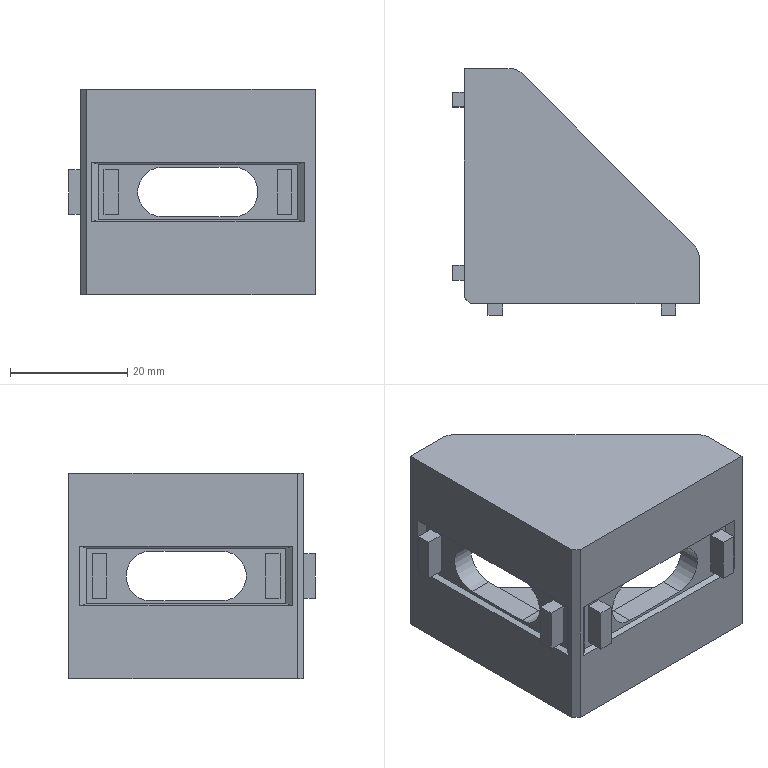Part | SolidWorks | features BaseBody 1 | 1 solid | 55 faces | box 42 x 42 x 35 mm | volume 15839 mm3 | plane 47 | cylinder 8 | commonest cylinder face diameters 6 x4 8.5 x4